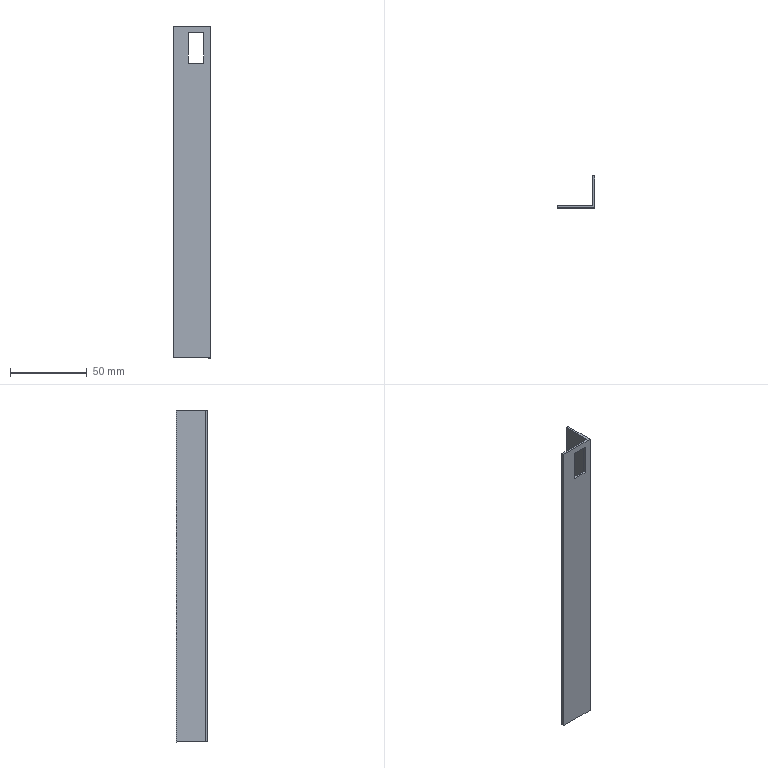Part | NX | features BREP 1 | 1 solid | 12 faces | box 24.5 x 20.5 x 216 mm | volume 13794 mm3 | plane 12
STEP:
#1=CARTESIAN_POINT('',(137.5,-105.,0.000000002));
#2=VERTEX_POINT('',#1);
#3=CARTESIAN_POINT('',(137.5,-103.5,0.000000002));
#4=VERTEX_POINT('',#3);
#5=CARTESIAN_POINT('',(137.5,-104.25,0.000000002));
#6=DIRECTION('',(0.,1.,0.));
#7=VECTOR('',#6,1000.);
#8=LINE('',#5,#7);
#9=EDGE_CURVE('',#2,#4,#8,.T.);
#10=ORIENTED_EDGE('',*,*,#9,.F.);
#11=CARTESIAN_POINT('',(137.5,-105.,216.));
#12=VERTEX_POINT('',#11);
#13=CARTESIAN_POINT('',(137.5,-105.,108.));
#14=DIRECTION('',(0.,0.,-1.));
#15=VECTOR('',#14,1000.);
#16=LINE('',#13,#15);
#17=EDGE_CURVE('',#12,#2,#16,.T.);
#18=ORIENTED_EDGE('',*,*,#17,.F.);
#19=CARTESIAN_POINT('',(137.5,-103.5,216.));
#20=VERTEX_POINT('',#19);
#21=CARTESIAN_POINT('',(137.5,-104.25,216.));
#22=DIRECTION('',(0.,1.,0.));
#23=VECTOR('',#22,1000.);
#24=LINE('',#21,#23);
#25=EDGE_CURVE('',#12,#20,#24,.T.);
#26=ORIENTED_EDGE('',*,*,#25,.T.);
#27=CARTESIAN_POINT('',(137.5,-103.5,108.));
#28=DIRECTION('',(0.,0.,-1.));
#29=VECTOR('',#28,1000.);
#30=LINE('',#27,#29);
#31=EDGE_CURVE('',#20,#4,#30,.T.);
#32=ORIENTED_EDGE('',*,*,#31,.T.);
#33=EDGE_LOOP('',(#10,#18,#26,#32));
#34=FACE_BOUND('',#33,.T.);
#35=CARTESIAN_POINT('',(137.5,-105.,216.));
#36=DIRECTION('',(1.,0.,0.));
#37=DIRECTION('',(0.,-1.,0.));
#38=AXIS2_PLACEMENT_3D('',#35,#36,#37);
#39=PLANE('',#38);
#40=ADVANCED_FACE('',(#34),#39,.F.);
#41=CARTESIAN_POINT('',(160.5,-84.5,0.000000002));
#42=VERTEX_POINT('',#41);
#43=CARTESIAN_POINT('',(162.,-84.5,0.000000002));
#44=VERTEX_POINT('',#43);
#45=CARTESIAN_POINT('',(161.25,-84.5,0.000000002));
#46=DIRECTION('',(1.,0.,0.));
#47=VECTOR('',#46,1000.);
#48=LINE('',#45,#47);
#49=EDGE_CURVE('',#42,#44,#48,.T.);
#50=ORIENTED_EDGE('',*,*,#49,.T.);
#51=CARTESIAN_POINT('',(162.,-105.,0.000000002));
#52=VERTEX_POINT('',#51);
#53=CARTESIAN_POINT('',(162.,-94.75,0.000000002));
#54=DIRECTION('',(0.,-1.,0.));
#55=VECTOR('',#54,1000.);
#56=LINE('',#53,#55);
#57=EDGE_CURVE('',#44,#52,#56,.T.);
#58=ORIENTED_EDGE('',*,*,#57,.T.);
#59=CARTESIAN_POINT('',(149.75,-105.,0.000000002));
#60=DIRECTION('',(-1.,0.,0.));
#61=VECTOR('',#60,1000.);
#62=LINE('',#59,#61);
#63=EDGE_CURVE('',#52,#2,#62,.T.);
#64=ORIENTED_EDGE('',*,*,#63,.T.);
#65=ORIENTED_EDGE('',*,*,#9,.T.);
#66=CARTESIAN_POINT('',(160.5,-103.5,0.000000002));
#67=VERTEX_POINT('',#66);
#68=CARTESIAN_POINT('',(149.,-103.5,0.000000002));
#69=DIRECTION('',(-1.,0.,0.));
#70=VECTOR('',#69,1000.);
#71=LINE('',#68,#70);
#72=EDGE_CURVE('',#67,#4,#71,.T.);
#73=ORIENTED_EDGE('',*,*,#72,.F.);
#74=CARTESIAN_POINT('',(160.5,-94.,0.000000002));
#75=DIRECTION('',(0.,-1.,0.));
#76=VECTOR('',#75,1000.);
#77=LINE('',#74,#76);
#78=EDGE_CURVE('',#42,#67,#77,.T.);
#79=ORIENTED_EDGE('',*,*,#78,.F.);
#80=EDGE_LOOP('',(#50,#58,#64,#65,#73,#79));
#81=FACE_BOUND('',#80,.T.);
#82=CARTESIAN_POINT('',(0.,212.,-0.000000001));
#83=DIRECTION('',(0.,0.,1.));
#84=DIRECTION('',(0.,1.,0.));
#85=AXIS2_PLACEMENT_3D('',#82,#83,#84);
#86=PLANE('',#85);
#87=ADVANCED_FACE('',(#81),#86,.F.);
#88=CARTESIAN_POINT('',(157.429,-105.,191.8));
#89=VERTEX_POINT('',#88);
#90=CARTESIAN_POINT('',(147.429,-105.,191.8));
#91=VERTEX_POINT('',#90);
#92=CARTESIAN_POINT('',(162.,-105.,191.8));
#93=DIRECTION('',(-1.,0.,0.));
#94=VECTOR('',#93,1000.);
#95=LINE('',#92,#94);
#96=EDGE_CURVE('',#89,#91,#95,.T.);
#97=ORIENTED_EDGE('',*,*,#96,.T.);
#98=CARTESIAN_POINT('',(147.429,-105.,211.8));
#99=VERTEX_POINT('',#98);
#100=CARTESIAN_POINT('',(147.429,-105.,216.));
#101=DIRECTION('',(0.,0.,1.));
#102=VECTOR('',#101,1000.);
#103=LINE('',#100,#102);
#104=EDGE_CURVE('',#91,#99,#103,.T.);
#105=ORIENTED_EDGE('',*,*,#104,.T.);
#106=CARTESIAN_POINT('',(157.429,-105.,211.8));
#107=VERTEX_POINT('',#106);
#108=CARTESIAN_POINT('',(162.,-105.,211.8));
#109=DIRECTION('',(1.,0.,0.));
#110=VECTOR('',#109,1000.);
#111=LINE('',#108,#110);
#112=EDGE_CURVE('',#99,#107,#111,.T.);
#113=ORIENTED_EDGE('',*,*,#112,.T.);
#114=CARTESIAN_POINT('',(157.429,-105.,216.));
#115=DIRECTION('',(0.,0.,-1.));
#116=VECTOR('',#115,1000.);
#117=LINE('',#114,#116);
#118=EDGE_CURVE('',#107,#89,#117,.T.);
#119=ORIENTED_EDGE('',*,*,#118,.T.);
#120=EDGE_LOOP('',(#97,#105,#113,#119));
#121=FACE_BOUND('',#120,.T.);
#122=CARTESIAN_POINT('',(162.,-105.,216.));
#123=VERTEX_POINT('',#122);
#124=CARTESIAN_POINT('',(162.,-105.,108.));
#125=DIRECTION('',(0.,0.,-1.));
#126=VECTOR('',#125,1000.);
#127=LINE('',#124,#126);
#128=EDGE_CURVE('',#123,#52,#127,.T.);
#129=ORIENTED_EDGE('',*,*,#128,.F.);
#130=CARTESIAN_POINT('',(149.75,-105.,216.));
#131=DIRECTION('',(-1.,0.,0.));
#132=VECTOR('',#131,1000.);
#133=LINE('',#130,#132);
#134=EDGE_CURVE('',#123,#12,#133,.T.);
#135=ORIENTED_EDGE('',*,*,#134,.T.);
#136=ORIENTED_EDGE('',*,*,#17,.T.);
#137=ORIENTED_EDGE('',*,*,#63,.F.);
#138=EDGE_LOOP('',(#129,#135,#136,#137));
#139=FACE_BOUND('',#138,.T.);
#140=CARTESIAN_POINT('',(162.,-105.,216.));
#141=DIRECTION('',(0.,1.,0.));
#142=DIRECTION('',(0.,0.,1.));
#143=AXIS2_PLACEMENT_3D('',#140,#141,#142);
#144=PLANE('',#143);
#145=ADVANCED_FACE('',(#121,#139),#144,.F.);
#146=CARTESIAN_POINT('',(160.5,-103.5,216.));
#147=VERTEX_POINT('',#146);
#148=CARTESIAN_POINT('',(149.,-103.5,216.));
#149=DIRECTION('',(-1.,0.,0.));
#150=VECTOR('',#149,1000.);
#151=LINE('',#148,#150);
#152=EDGE_CURVE('',#147,#20,#151,.T.);
#153=ORIENTED_EDGE('',*,*,#152,.T.);
#154=ORIENTED_EDGE('',*,*,#25,.F.);
#155=ORIENTED_EDGE('',*,*,#134,.F.);
#156=CARTESIAN_POINT('',(162.,-84.5,216.));
#157=VERTEX_POINT('',#156);
#158=CARTESIAN_POINT('',(162.,-94.75,216.));
#159=DIRECTION('',(0.,-1.,0.));
#160=VECTOR('',#159,1000.);
#161=LINE('',#158,#160);
#162=EDGE_CURVE('',#157,#123,#161,.T.);
#163=ORIENTED_EDGE('',*,*,#162,.F.);
#164=CARTESIAN_POINT('',(160.5,-84.5,216.));
#165=VERTEX_POINT('',#164);
#166=CARTESIAN_POINT('',(161.25,-84.5,216.));
#167=DIRECTION('',(1.,0.,0.));
#168=VECTOR('',#167,1000.);
#169=LINE('',#166,#168);
#170=EDGE_CURVE('',#165,#157,#169,.T.);
#171=ORIENTED_EDGE('',*,*,#170,.F.);
#172=CARTESIAN_POINT('',(160.5,-94.,216.));
#173=DIRECTION('',(0.,-1.,0.));
#174=VECTOR('',#173,1000.);
#175=LINE('',#172,#174);
#176=EDGE_CURVE('',#165,#147,#175,.T.);
#177=ORIENTED_EDGE('',*,*,#176,.T.);
#178=EDGE_LOOP('',(#153,#154,#155,#163,#171,#177));
#179=FACE_BOUND('',#178,.T.);
#180=CARTESIAN_POINT('',(0.,212.,216.));
#181=DIRECTION('',(0.,0.,1.));
#182=DIRECTION('',(0.,1.,0.));
#183=AXIS2_PLACEMENT_3D('',#180,#181,#182);
#184=PLANE('',#183);
#185=ADVANCED_FACE('',(#179),#184,.T.);
#186=CARTESIAN_POINT('',(147.429,-103.5,191.8));
#187=VERTEX_POINT('',#186);
#188=CARTESIAN_POINT('',(147.429,-103.5,211.8));
#189=VERTEX_POINT('',#188);
#190=CARTESIAN_POINT('',(147.429,-103.5,191.8));
#191=DIRECTION('',(0.,0.,1.));
#192=VECTOR('',#191,1000.);
#193=LINE('',#190,#192);
#194=EDGE_CURVE('',#187,#189,#193,.T.);
#195=ORIENTED_EDGE('',*,*,#194,.F.);
#196=CARTESIAN_POINT('',(157.429,-103.5,191.8));
#197=VERTEX_POINT('',#196);
#198=CARTESIAN_POINT('',(157.429,-103.5,191.8));
#199=DIRECTION('',(-1.,0.,0.));
#200=VECTOR('',#199,1000.);
#201=LINE('',#198,#200);
#202=EDGE_CURVE('',#197,#187,#201,.T.);
#203=ORIENTED_EDGE('',*,*,#202,.F.);
#204=CARTESIAN_POINT('',(157.429,-103.5,211.8));
#205=VERTEX_POINT('',#204);
#206=CARTESIAN_POINT('',(157.429,-103.5,211.8));
#207=DIRECTION('',(0.,0.,-1.));
#208=VECTOR('',#207,1000.);
#209=LINE('',#206,#208);
#210=EDGE_CURVE('',#205,#197,#209,.T.);
#211=ORIENTED_EDGE('',*,*,#210,.F.);
#212=CARTESIAN_POINT('',(147.429,-103.5,211.8));
#213=DIRECTION('',(1.,0.,0.));
#214=VECTOR('',#213,1000.);
#215=LINE('',#212,#214);
#216=EDGE_CURVE('',#189,#205,#215,.T.);
#217=ORIENTED_EDGE('',*,*,#216,.F.);
#218=EDGE_LOOP('',(#195,#203,#211,#217));
#219=FACE_BOUND('',#218,.T.);
#220=ORIENTED_EDGE('',*,*,#31,.F.);
#221=ORIENTED_EDGE('',*,*,#152,.F.);
#222=CARTESIAN_POINT('',(160.5,-103.5,108.));
#223=DIRECTION('',(0.,0.,-1.));
#224=VECTOR('',#223,1000.);
#225=LINE('',#222,#224);
#226=EDGE_CURVE('',#147,#67,#225,.T.);
#227=ORIENTED_EDGE('',*,*,#226,.T.);
#228=ORIENTED_EDGE('',*,*,#72,.T.);
#229=EDGE_LOOP('',(#220,#221,#227,#228));
#230=FACE_BOUND('',#229,.T.);
#231=CARTESIAN_POINT('',(162.,-103.5,216.));
#232=DIRECTION('',(0.,1.,0.));
#233=DIRECTION('',(0.,0.,1.));
#234=AXIS2_PLACEMENT_3D('',#231,#232,#233);
#235=PLANE('',#234);
#236=ADVANCED_FACE('',(#219,#230),#235,.T.);
#237=CARTESIAN_POINT('',(162.,-84.5,108.));
#238=DIRECTION('',(0.,0.,-1.));
#239=VECTOR('',#238,1000.);
#240=LINE('',#237,#239);
#241=EDGE_CURVE('',#157,#44,#240,.T.);
#242=ORIENTED_EDGE('',*,*,#241,.T.);
#243=ORIENTED_EDGE('',*,*,#49,.F.);
#244=CARTESIAN_POINT('',(160.5,-84.5,108.));
#245=DIRECTION('',(0.,0.,-1.));
#246=VECTOR('',#245,1000.);
#247=LINE('',#244,#246);
#248=EDGE_CURVE('',#165,#42,#247,.T.);
#249=ORIENTED_EDGE('',*,*,#248,.F.);
#250=ORIENTED_EDGE('',*,*,#170,.T.);
#251=EDGE_LOOP('',(#242,#243,#249,#250));
#252=FACE_BOUND('',#251,.T.);
#253=CARTESIAN_POINT('',(137.5,-84.5,216.));
#254=DIRECTION('',(0.,-1.,0.));
#255=DIRECTION('',(1.,0.,0.));
#256=AXIS2_PLACEMENT_3D('',#253,#254,#255);
#257=PLANE('',#256);
#258=ADVANCED_FACE('',(#252),#257,.F.);
#259=ORIENTED_EDGE('',*,*,#241,.F.);
#260=ORIENTED_EDGE('',*,*,#162,.T.);
#261=ORIENTED_EDGE('',*,*,#128,.T.);
#262=ORIENTED_EDGE('',*,*,#57,.F.);
#263=EDGE_LOOP('',(#259,#260,#261,#262));
#264=FACE_BOUND('',#263,.T.);
#265=CARTESIAN_POINT('',(162.,-84.5,216.));
#266=DIRECTION('',(-1.,0.,0.));
#267=DIRECTION('',(0.,0.,-1.));
#268=AXIS2_PLACEMENT_3D('',#265,#266,#267);
#269=PLANE('',#268);
#270=ADVANCED_FACE('',(#264),#269,.F.);
#271=ORIENTED_EDGE('',*,*,#226,.F.);
#272=ORIENTED_EDGE('',*,*,#176,.F.);
#273=ORIENTED_EDGE('',*,*,#248,.T.);
#274=ORIENTED_EDGE('',*,*,#78,.T.);
#275=EDGE_LOOP('',(#271,#272,#273,#274));
#276=FACE_BOUND('',#275,.T.);
#277=CARTESIAN_POINT('',(160.5,-84.5,216.));
#278=DIRECTION('',(-1.,0.,0.));
#279=DIRECTION('',(0.,0.,-1.));
#280=AXIS2_PLACEMENT_3D('',#277,#278,#279);
#281=PLANE('',#280);
#282=ADVANCED_FACE('',(#276),#281,.T.);
#283=CARTESIAN_POINT('',(147.429,-111.,191.8));
#284=DIRECTION('',(0.,-1.,0.));
#285=VECTOR('',#284,1000.);
#286=LINE('',#283,#285);
#287=EDGE_CURVE('',#187,#91,#286,.T.);
#288=ORIENTED_EDGE('',*,*,#287,.F.);
#289=ORIENTED_EDGE('',*,*,#194,.T.);
#290=CARTESIAN_POINT('',(147.429,-111.,211.8));
#291=DIRECTION('',(0.,-1.,0.));
#292=VECTOR('',#291,1000.);
#293=LINE('',#290,#292);
#294=EDGE_CURVE('',#189,#99,#293,.T.);
#295=ORIENTED_EDGE('',*,*,#294,.T.);
#296=ORIENTED_EDGE('',*,*,#104,.F.);
#297=EDGE_LOOP('',(#288,#289,#295,#296));
#298=FACE_BOUND('',#297,.T.);
#299=CARTESIAN_POINT('',(147.429,-111.,191.8));
#300=DIRECTION('',(-1.,0.,0.));
#301=DIRECTION('',(0.,0.,-1.));
#302=AXIS2_PLACEMENT_3D('',#299,#300,#301);
#303=PLANE('',#302);
#304=ADVANCED_FACE('',(#298),#303,.F.);
#305=ORIENTED_EDGE('',*,*,#294,.F.);
#306=ORIENTED_EDGE('',*,*,#216,.T.);
#307=CARTESIAN_POINT('',(157.429,-111.,211.8));
#308=DIRECTION('',(0.,-1.,0.));
#309=VECTOR('',#308,1000.);
#310=LINE('',#307,#309);
#311=EDGE_CURVE('',#205,#107,#310,.T.);
#312=ORIENTED_EDGE('',*,*,#311,.T.);
#313=ORIENTED_EDGE('',*,*,#112,.F.);
#314=EDGE_LOOP('',(#305,#306,#312,#313));
#315=FACE_BOUND('',#314,.T.);
#316=CARTESIAN_POINT('',(147.429,-111.,211.8));
#317=DIRECTION('',(0.,0.,1.));
#318=DIRECTION('',(-1.,0.,0.));
#319=AXIS2_PLACEMENT_3D('',#316,#317,#318);
#320=PLANE('',#319);
#321=ADVANCED_FACE('',(#315),#320,.F.);
#322=ORIENTED_EDGE('',*,*,#311,.F.);
#323=ORIENTED_EDGE('',*,*,#210,.T.);
#324=CARTESIAN_POINT('',(157.429,-111.,191.8));
#325=DIRECTION('',(0.,-1.,0.));
#326=VECTOR('',#325,1000.);
#327=LINE('',#324,#326);
#328=EDGE_CURVE('',#197,#89,#327,.T.);
#329=ORIENTED_EDGE('',*,*,#328,.T.);
#330=ORIENTED_EDGE('',*,*,#118,.F.);
#331=EDGE_LOOP('',(#322,#323,#329,#330));
#332=FACE_BOUND('',#331,.T.);
#333=CARTESIAN_POINT('',(157.429,-111.,211.8));
#334=DIRECTION('',(1.,0.,0.));
#335=DIRECTION('',(0.,0.,1.));
#336=AXIS2_PLACEMENT_3D('',#333,#334,#335);
#337=PLANE('',#336);
#338=ADVANCED_FACE('',(#332),#337,.F.);
#339=ORIENTED_EDGE('',*,*,#328,.F.);
#340=ORIENTED_EDGE('',*,*,#202,.T.);
#341=ORIENTED_EDGE('',*,*,#287,.T.);
#342=ORIENTED_EDGE('',*,*,#96,.F.);
#343=EDGE_LOOP('',(#339,#340,#341,#342));
#344=FACE_BOUND('',#343,.T.);
#345=CARTESIAN_POINT('',(157.429,-111.,191.8));
#346=DIRECTION('',(0.,0.,-1.));
#347=DIRECTION('',(1.,0.,0.));
#348=AXIS2_PLACEMENT_3D('',#345,#346,#347);
#349=PLANE('',#348);
#350=ADVANCED_FACE('',(#344),#349,.F.);
#351=CLOSED_SHELL('',(#40,#87,#145,#185,#236,#258,#270,#282,#304,#321,#338,#350));
#352=MANIFOLD_SOLID_BREP('',#351);
#353=(LENGTH_UNIT()NAMED_UNIT(*)SI_UNIT(.MILLI.,.METRE.));
#354=UNCERTAINTY_MEASURE_WITH_UNIT(LENGTH_MEASURE(0.00001),#353,'','');
#355=(NAMED_UNIT(*)PLANE_ANGLE_UNIT()SI_UNIT($,.RADIAN.));
#356=(NAMED_UNIT(*)SI_UNIT($,.STERADIAN.)SOLID_ANGLE_UNIT());
#357=(GEOMETRIC_REPRESENTATION_CONTEXT(3)GLOBAL_UNCERTAINTY_ASSIGNED_CONTEXT((#354))GLOBAL_UNIT_ASSIGNED_CONTEXT((#353,#355,#356))REPRESENTATION_CONTEXT('',''));
#358=ADVANCED_BREP_SHAPE_REPRESENTATION('',(#352),#357);